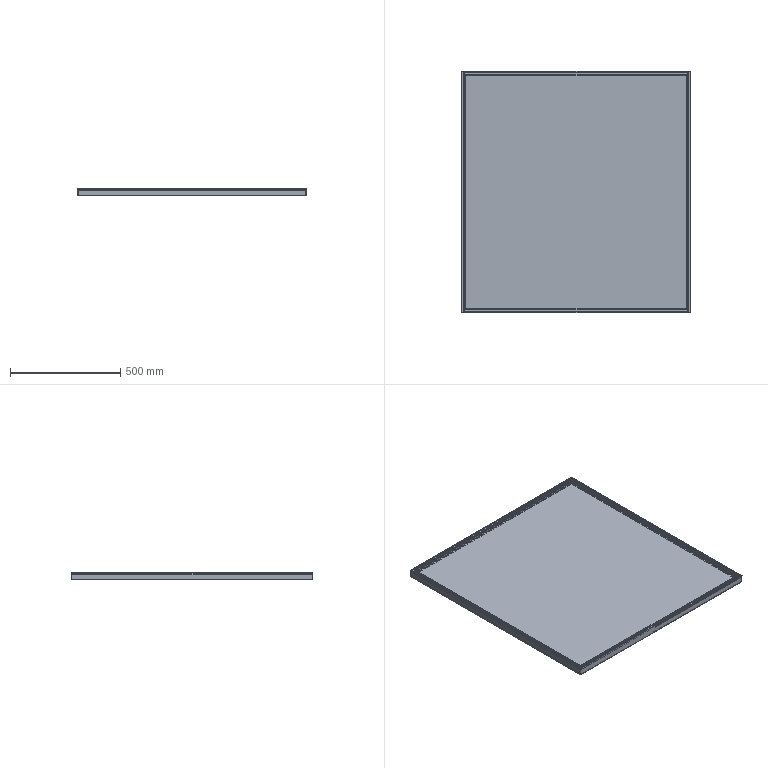Part | SolidWorks | features ICE 1, WeldMemberFeat 1, WeldmentFeature 1 | 5 solids | 94 faces | box 1035 x 1095 x 35 mm | volume 3941366 mm3 | plane 86 | cylinder 8 | commonest cylinder face diameters 1 x4 2 x4